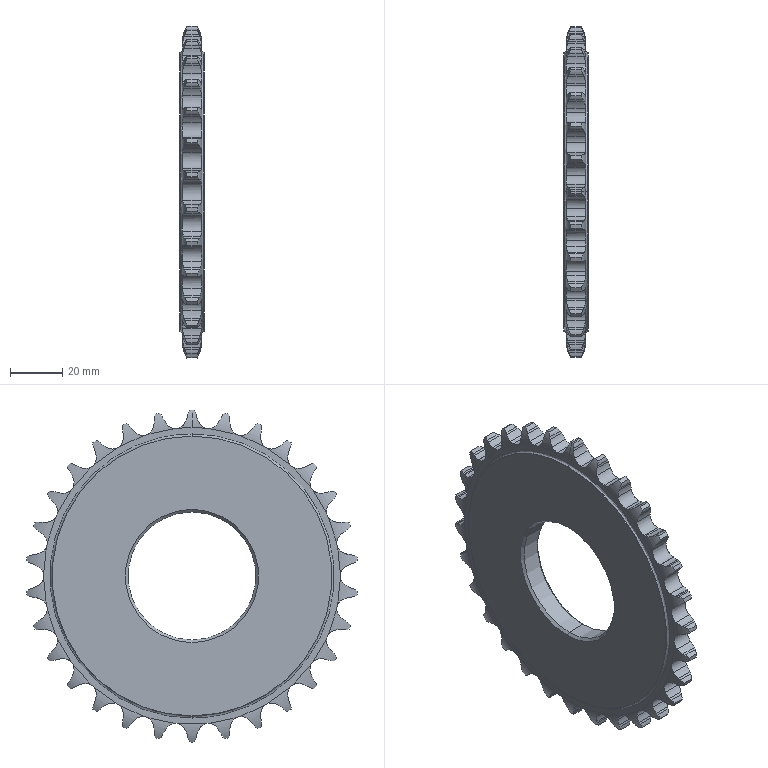Part | STEP file | PN_0043_driving sprocket_05B | 1 solid | 337 faces | box 9.37 x 126.465 x 127 mm | volume 80983 mm3 | cylinder 203 | spline 66 | plane 64 | cone 4 | commonest cylinder face diameters 11.344 x64 20.732 x64 8.06 x38 127 x31 107 x4 49 x2